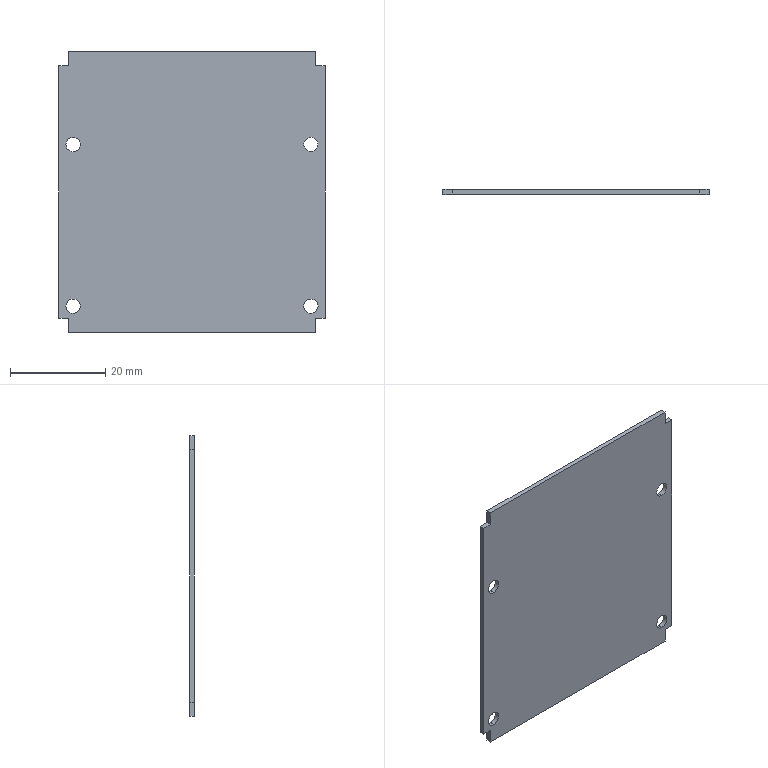Part | NX | features BREP 1 | 1 solid | 22 faces | box 56 x 1 x 59 mm | volume 3252 mm3 | plane 14 | cylinder 8 | commonest cylinder face diameters 3 x8
STEP:
#1=CARTESIAN_POINT('',(25.,1.,8.5));
#2=VERTEX_POINT('',#1);
#3=CARTESIAN_POINT('',(25.,1.,11.5));
#4=VERTEX_POINT('',#3);
#5=CARTESIAN_POINT('',(25.,1.,10.));
#6=DIRECTION('',(0.,1.,0.));
#7=DIRECTION('',(1.,0.,0.));
#8=AXIS2_PLACEMENT_3D('',#5,#6,#7);
#9=CIRCLE('',#8,1.5);
#10=EDGE_CURVE('',#2,#4,#9,.T.);
#11=ORIENTED_EDGE('',*,*,#10,.T.);
#12=CARTESIAN_POINT('',(25.,0.,11.5));
#13=VERTEX_POINT('',#12);
#14=CARTESIAN_POINT('',(25.,1.,11.5));
#15=DIRECTION('',(0.,1.,0.));
#16=VECTOR('',#15,1000.);
#17=LINE('',#14,#16);
#18=EDGE_CURVE('',#13,#4,#17,.T.);
#19=ORIENTED_EDGE('',*,*,#18,.F.);
#20=CARTESIAN_POINT('',(25.,0.,8.5));
#21=VERTEX_POINT('',#20);
#22=CARTESIAN_POINT('',(25.,0.,10.));
#23=DIRECTION('',(0.,1.,0.));
#24=DIRECTION('',(1.,0.,0.));
#25=AXIS2_PLACEMENT_3D('',#22,#23,#24);
#26=CIRCLE('',#25,1.5);
#27=EDGE_CURVE('',#21,#13,#26,.T.);
#28=ORIENTED_EDGE('',*,*,#27,.F.);
#29=CARTESIAN_POINT('',(25.,1.,8.5));
#30=DIRECTION('',(0.,1.,0.));
#31=VECTOR('',#30,1000.);
#32=LINE('',#29,#31);
#33=EDGE_CURVE('',#21,#2,#32,.T.);
#34=ORIENTED_EDGE('',*,*,#33,.T.);
#35=EDGE_LOOP('',(#11,#19,#28,#34));
#36=FACE_BOUND('',#35,.T.);
#37=CARTESIAN_POINT('',(25.,1.,10.));
#38=DIRECTION('',(0.,-1.,0.));
#39=DIRECTION('',(0.,0.,-1.));
#40=AXIS2_PLACEMENT_3D('',#37,#38,#39);
#41=CYLINDRICAL_SURFACE('',#40,1.5);
#42=ADVANCED_FACE('',(#36),#41,.F.);
#43=CARTESIAN_POINT('',(28.,1.,26.5));
#44=VERTEX_POINT('',#43);
#45=CARTESIAN_POINT('',(28.,1.,-26.5));
#46=VERTEX_POINT('',#45);
#47=CARTESIAN_POINT('',(28.,1.,0.));
#48=DIRECTION('',(0.,0.,-1.));
#49=VECTOR('',#48,1000.);
#50=LINE('',#47,#49);
#51=EDGE_CURVE('',#44,#46,#50,.T.);
#52=ORIENTED_EDGE('',*,*,#51,.T.);
#53=CARTESIAN_POINT('',(26.,1.,-26.5));
#54=VERTEX_POINT('',#53);
#55=CARTESIAN_POINT('',(27.,1.,-26.5));
#56=DIRECTION('',(-1.,0.,0.));
#57=VECTOR('',#56,1000.);
#58=LINE('',#55,#57);
#59=EDGE_CURVE('',#46,#54,#58,.T.);
#60=ORIENTED_EDGE('',*,*,#59,.T.);
#61=CARTESIAN_POINT('',(26.,1.,-29.5));
#62=VERTEX_POINT('',#61);
#63=CARTESIAN_POINT('',(26.,1.,-28.));
#64=DIRECTION('',(0.,0.,-1.));
#65=VECTOR('',#64,1000.);
#66=LINE('',#63,#65);
#67=EDGE_CURVE('',#54,#62,#66,.T.);
#68=ORIENTED_EDGE('',*,*,#67,.T.);
#69=CARTESIAN_POINT('',(-26.,1.,-29.5));
#70=VERTEX_POINT('',#69);
#71=CARTESIAN_POINT('',(0.,1.,-29.5));
#72=DIRECTION('',(-1.,0.,0.));
#73=VECTOR('',#72,1000.);
#74=LINE('',#71,#73);
#75=EDGE_CURVE('',#62,#70,#74,.T.);
#76=ORIENTED_EDGE('',*,*,#75,.T.);
#77=CARTESIAN_POINT('',(-26.,1.,-26.5));
#78=VERTEX_POINT('',#77);
#79=CARTESIAN_POINT('',(-26.,1.,-28.));
#80=DIRECTION('',(0.,0.,1.));
#81=VECTOR('',#80,1000.);
#82=LINE('',#79,#81);
#83=EDGE_CURVE('',#70,#78,#82,.T.);
#84=ORIENTED_EDGE('',*,*,#83,.T.);
#85=CARTESIAN_POINT('',(-28.,1.,-26.5));
#86=VERTEX_POINT('',#85);
#87=CARTESIAN_POINT('',(-27.,1.,-26.5));
#88=DIRECTION('',(-1.,0.,0.));
#89=VECTOR('',#88,1000.);
#90=LINE('',#87,#89);
#91=EDGE_CURVE('',#78,#86,#90,.T.);
#92=ORIENTED_EDGE('',*,*,#91,.T.);
#93=CARTESIAN_POINT('',(-28.,1.,26.5));
#94=VERTEX_POINT('',#93);
#95=CARTESIAN_POINT('',(-28.,1.,0.));
#96=DIRECTION('',(0.,0.,1.));
#97=VECTOR('',#96,1000.);
#98=LINE('',#95,#97);
#99=EDGE_CURVE('',#86,#94,#98,.T.);
#100=ORIENTED_EDGE('',*,*,#99,.T.);
#101=CARTESIAN_POINT('',(-26.,1.,26.5));
#102=VERTEX_POINT('',#101);
#103=CARTESIAN_POINT('',(-27.,1.,26.5));
#104=DIRECTION('',(1.,0.,0.));
#105=VECTOR('',#104,1000.);
#106=LINE('',#103,#105);
#107=EDGE_CURVE('',#94,#102,#106,.T.);
#108=ORIENTED_EDGE('',*,*,#107,.T.);
#109=CARTESIAN_POINT('',(-26.,1.,29.5));
#110=VERTEX_POINT('',#109);
#111=CARTESIAN_POINT('',(-26.,1.,28.));
#112=DIRECTION('',(0.,0.,1.));
#113=VECTOR('',#112,1000.);
#114=LINE('',#111,#113);
#115=EDGE_CURVE('',#102,#110,#114,.T.);
#116=ORIENTED_EDGE('',*,*,#115,.T.);
#117=CARTESIAN_POINT('',(26.,1.,29.5));
#118=VERTEX_POINT('',#117);
#119=CARTESIAN_POINT('',(0.,1.,29.5));
#120=DIRECTION('',(1.,0.,0.));
#121=VECTOR('',#120,1000.);
#122=LINE('',#119,#121);
#123=EDGE_CURVE('',#110,#118,#122,.T.);
#124=ORIENTED_EDGE('',*,*,#123,.T.);
#125=CARTESIAN_POINT('',(26.,1.,26.5));
#126=VERTEX_POINT('',#125);
#127=CARTESIAN_POINT('',(26.,1.,28.));
#128=DIRECTION('',(0.,0.,-1.));
#129=VECTOR('',#128,1000.);
#130=LINE('',#127,#129);
#131=EDGE_CURVE('',#118,#126,#130,.T.);
#132=ORIENTED_EDGE('',*,*,#131,.T.);
#133=CARTESIAN_POINT('',(27.,1.,26.5));
#134=DIRECTION('',(1.,0.,0.));
#135=VECTOR('',#134,1000.);
#136=LINE('',#133,#135);
#137=EDGE_CURVE('',#126,#44,#136,.T.);
#138=ORIENTED_EDGE('',*,*,#137,.T.);
#139=EDGE_LOOP('',(#52,#60,#68,#76,#84,#92,#100,#108,#116,#124,#132,#138));
#140=FACE_BOUND('',#139,.T.);
#141=CARTESIAN_POINT('',(-25.,1.,-25.5));
#142=VERTEX_POINT('',#141);
#143=CARTESIAN_POINT('',(-25.,1.,-22.5));
#144=VERTEX_POINT('',#143);
#145=CARTESIAN_POINT('',(-25.,1.,-25.5));
#146=CARTESIAN_POINT('',(-25.18,1.,-25.5));
#147=CARTESIAN_POINT('',(-25.36,1.,-25.473));
#148=CARTESIAN_POINT('',(-25.535,1.,-25.419));
#149=CARTESIAN_POINT('',(-25.862,1.,-25.26));
#150=CARTESIAN_POINT('',(-26.129,1.,-25.012));
#151=CARTESIAN_POINT('',(-26.242,1.,-24.869));
#152=CARTESIAN_POINT('',(-26.423,1.,-24.553));
#153=CARTESIAN_POINT('',(-26.503,1.,-24.198));
#154=CARTESIAN_POINT('',(-26.516,1.,-24.016));
#155=CARTESIAN_POINT('',(-26.487,1.,-23.653));
#156=CARTESIAN_POINT('',(-26.353,1.,-23.315));
#157=CARTESIAN_POINT('',(-26.26,1.,-23.157));
#158=CARTESIAN_POINT('',(-26.031,1.,-22.874));
#159=CARTESIAN_POINT('',(-25.73,1.,-22.671));
#160=CARTESIAN_POINT('',(-25.564,1.,-22.593));
#161=CARTESIAN_POINT('',(-25.349,1.,-22.528));
#162=CARTESIAN_POINT('',(-25.127,1.,-22.505));
#163=CARTESIAN_POINT('',(-25.085,1.,-22.502));
#164=CARTESIAN_POINT('',(-25.042,1.,-22.5));
#165=CARTESIAN_POINT('',(-25.,1.,-22.5));
#166=B_SPLINE_CURVE_WITH_KNOTS('',5,(#145,#146,#147,#148,#149,#150,#151,#152,#153,#154,#155,#156,#157,#158,#159,#160,#161,#162,#163,#164,#165),.UNSPECIFIED.,.F.,.F.,(6,3,3,3,3,3,6),(0.,0.191,0.382,0.573,0.764,0.9549,1.),.UNSPECIFIED.);
#167=EDGE_CURVE('',#142,#144,#166,.T.);
#168=ORIENTED_EDGE('',*,*,#167,.F.);
#169=CARTESIAN_POINT('',(-25.,1.,-22.5));
#170=CARTESIAN_POINT('',(-24.82,1.,-22.5));
#171=CARTESIAN_POINT('',(-24.64,1.,-22.527));
#172=CARTESIAN_POINT('',(-24.465,1.,-22.581));
#173=CARTESIAN_POINT('',(-24.138,1.,-22.74));
#174=CARTESIAN_POINT('',(-23.871,1.,-22.988));
#175=CARTESIAN_POINT('',(-23.758,1.,-23.131));
#176=CARTESIAN_POINT('',(-23.577,1.,-23.447));
#177=CARTESIAN_POINT('',(-23.497,1.,-23.802));
#178=CARTESIAN_POINT('',(-23.484,1.,-23.984));
#179=CARTESIAN_POINT('',(-23.513,1.,-24.347));
#180=CARTESIAN_POINT('',(-23.647,1.,-24.685));
#181=CARTESIAN_POINT('',(-23.74,1.,-24.843));
#182=CARTESIAN_POINT('',(-23.969,1.,-25.126));
#183=CARTESIAN_POINT('',(-24.27,1.,-25.329));
#184=CARTESIAN_POINT('',(-24.436,1.,-25.407));
#185=CARTESIAN_POINT('',(-24.651,1.,-25.472));
#186=CARTESIAN_POINT('',(-24.873,1.,-25.495));
#187=CARTESIAN_POINT('',(-24.915,1.,-25.498));
#188=CARTESIAN_POINT('',(-24.958,1.,-25.5));
#189=CARTESIAN_POINT('',(-25.,1.,-25.5));
#190=B_SPLINE_CURVE_WITH_KNOTS('',5,(#169,#170,#171,#172,#173,#174,#175,#176,#177,#178,#179,#180,#181,#182,#183,#184,#185,#186,#187,#188,#189),.UNSPECIFIED.,.F.,.F.,(6,3,3,3,3,3,6),(0.,0.191,0.382,0.573,0.764,0.9549,1.),.UNSPECIFIED.);
#191=EDGE_CURVE('',#144,#142,#190,.T.);
#192=ORIENTED_EDGE('',*,*,#191,.F.);
#193=EDGE_LOOP('',(#168,#192));
#194=FACE_BOUND('',#193,.T.);
#195=CARTESIAN_POINT('',(25.,1.,-25.5));
#196=VERTEX_POINT('',#195);
#197=CARTESIAN_POINT('',(25.,1.,-22.5));
#198=VERTEX_POINT('',#197);
#199=CARTESIAN_POINT('',(25.,1.,-25.5));
#200=CARTESIAN_POINT('',(24.82,1.,-25.5));
#201=CARTESIAN_POINT('',(24.64,1.,-25.473));
#202=CARTESIAN_POINT('',(24.465,1.,-25.419));
#203=CARTESIAN_POINT('',(24.138,1.,-25.26));
#204=CARTESIAN_POINT('',(23.871,1.,-25.012));
#205=CARTESIAN_POINT('',(23.758,1.,-24.869));
#206=CARTESIAN_POINT('',(23.577,1.,-24.553));
#207=CARTESIAN_POINT('',(23.497,1.,-24.198));
#208=CARTESIAN_POINT('',(23.484,1.,-24.016));
#209=CARTESIAN_POINT('',(23.513,1.,-23.653));
#210=CARTESIAN_POINT('',(23.647,1.,-23.315));
#211=CARTESIAN_POINT('',(23.74,1.,-23.157));
#212=CARTESIAN_POINT('',(23.969,1.,-22.874));
#213=CARTESIAN_POINT('',(24.27,1.,-22.671));
#214=CARTESIAN_POINT('',(24.436,1.,-22.593));
#215=CARTESIAN_POINT('',(24.651,1.,-22.528));
#216=CARTESIAN_POINT('',(24.873,1.,-22.505));
#217=CARTESIAN_POINT('',(24.915,1.,-22.502));
#218=CARTESIAN_POINT('',(24.958,1.,-22.5));
#219=CARTESIAN_POINT('',(25.,1.,-22.5));
#220=B_SPLINE_CURVE_WITH_KNOTS('',5,(#199,#200,#201,#202,#203,#204,#205,#206,#207,#208,#209,#210,#211,#212,#213,#214,#215,#216,#217,#218,#219),.UNSPECIFIED.,.F.,.F.,(6,3,3,3,3,3,6),(0.,0.191,0.382,0.573,0.764,0.9549,1.),.UNSPECIFIED.);
#221=EDGE_CURVE('',#196,#198,#220,.T.);
#222=ORIENTED_EDGE('',*,*,#221,.F.);
#223=CARTESIAN_POINT('',(25.,1.,-22.5));
#224=CARTESIAN_POINT('',(25.18,1.,-22.5));
#225=CARTESIAN_POINT('',(25.36,1.,-22.527));
#226=CARTESIAN_POINT('',(25.535,1.,-22.581));
#227=CARTESIAN_POINT('',(25.862,1.,-22.74));
#228=CARTESIAN_POINT('',(26.129,1.,-22.988));
#229=CARTESIAN_POINT('',(26.242,1.,-23.131));
#230=CARTESIAN_POINT('',(26.423,1.,-23.447));
#231=CARTESIAN_POINT('',(26.503,1.,-23.802));
#232=CARTESIAN_POINT('',(26.516,1.,-23.984));
#233=CARTESIAN_POINT('',(26.487,1.,-24.347));
#234=CARTESIAN_POINT('',(26.353,1.,-24.685));
#235=CARTESIAN_POINT('',(26.26,1.,-24.843));
#236=CARTESIAN_POINT('',(26.031,1.,-25.126));
#237=CARTESIAN_POINT('',(25.73,1.,-25.329));
#238=CARTESIAN_POINT('',(25.564,1.,-25.407));
#239=CARTESIAN_POINT('',(25.349,1.,-25.472));
#240=CARTESIAN_POINT('',(25.127,1.,-25.495));
#241=CARTESIAN_POINT('',(25.085,1.,-25.498));
#242=CARTESIAN_POINT('',(25.042,1.,-25.5));
#243=CARTESIAN_POINT('',(25.,1.,-25.5));
#244=B_SPLINE_CURVE_WITH_KNOTS('',5,(#223,#224,#225,#226,#227,#228,#229,#230,#231,#232,#233,#234,#235,#236,#237,#238,#239,#240,#241,#242,#243),.UNSPECIFIED.,.F.,.F.,(6,3,3,3,3,3,6),(0.,0.191,0.382,0.573,0.764,0.9549,1.),.UNSPECIFIED.);
#245=EDGE_CURVE('',#198,#196,#244,.T.);
#246=ORIENTED_EDGE('',*,*,#245,.F.);
#247=EDGE_LOOP('',(#222,#246));
#248=FACE_BOUND('',#247,.T.);
#249=CARTESIAN_POINT('',(-25.,1.,8.5));
#250=VERTEX_POINT('',#249);
#251=CARTESIAN_POINT('',(-25.,1.,11.5));
#252=VERTEX_POINT('',#251);
#253=CARTESIAN_POINT('',(-25.,1.,8.5));
#254=CARTESIAN_POINT('',(-25.18,1.,8.5));
#255=CARTESIAN_POINT('',(-25.36,1.,8.527));
#256=CARTESIAN_POINT('',(-25.535,1.,8.581));
#257=CARTESIAN_POINT('',(-25.862,1.,8.74));
#258=CARTESIAN_POINT('',(-26.129,1.,8.988));
#259=CARTESIAN_POINT('',(-26.242,1.,9.131));
#260=CARTESIAN_POINT('',(-26.423,1.,9.447));
#261=CARTESIAN_POINT('',(-26.503,1.,9.802));
#262=CARTESIAN_POINT('',(-26.516,1.,9.984));
#263=CARTESIAN_POINT('',(-26.487,1.,10.347));
#264=CARTESIAN_POINT('',(-26.353,1.,10.685));
#265=CARTESIAN_POINT('',(-26.26,1.,10.843));
#266=CARTESIAN_POINT('',(-26.031,1.,11.126));
#267=CARTESIAN_POINT('',(-25.73,1.,11.329));
#268=CARTESIAN_POINT('',(-25.564,1.,11.407));
#269=CARTESIAN_POINT('',(-25.349,1.,11.472));
#270=CARTESIAN_POINT('',(-25.127,1.,11.495));
#271=CARTESIAN_POINT('',(-25.085,1.,11.498));
#272=CARTESIAN_POINT('',(-25.042,1.,11.5));
#273=CARTESIAN_POINT('',(-25.,1.,11.5));
#274=B_SPLINE_CURVE_WITH_KNOTS('',5,(#253,#254,#255,#256,#257,#258,#259,#260,#261,#262,#263,#264,#265,#266,#267,#268,#269,#270,#271,#272,#273),.UNSPECIFIED.,.F.,.F.,(6,3,3,3,3,3,6),(0.,0.191,0.382,0.573,0.764,0.9549,1.),.UNSPECIFIED.);
#275=EDGE_CURVE('',#250,#252,#274,.T.);
#276=ORIENTED_EDGE('',*,*,#275,.F.);
#277=CARTESIAN_POINT('',(-25.,1.,11.5));
#278=CARTESIAN_POINT('',(-24.82,1.,11.5));
#279=CARTESIAN_POINT('',(-24.64,1.,11.473));
#280=CARTESIAN_POINT('',(-24.465,1.,11.419));
#281=CARTESIAN_POINT('',(-24.138,1.,11.26));
#282=CARTESIAN_POINT('',(-23.871,1.,11.012));
#283=CARTESIAN_POINT('',(-23.758,1.,10.869));
#284=CARTESIAN_POINT('',(-23.577,1.,10.553));
#285=CARTESIAN_POINT('',(-23.497,1.,10.198));
#286=CARTESIAN_POINT('',(-23.484,1.,10.016));
#287=CARTESIAN_POINT('',(-23.513,1.,9.653));
#288=CARTESIAN_POINT('',(-23.647,1.,9.315));
#289=CARTESIAN_POINT('',(-23.74,1.,9.157));
#290=CARTESIAN_POINT('',(-23.969,1.,8.874));
#291=CARTESIAN_POINT('',(-24.27,1.,8.671));
#292=CARTESIAN_POINT('',(-24.436,1.,8.593));
#293=CARTESIAN_POINT('',(-24.651,1.,8.528));
#294=CARTESIAN_POINT('',(-24.873,1.,8.505));
#295=CARTESIAN_POINT('',(-24.915,1.,8.502));
#296=CARTESIAN_POINT('',(-24.958,1.,8.5));
#297=CARTESIAN_POINT('',(-25.,1.,8.5));
#298=B_SPLINE_CURVE_WITH_KNOTS('',5,(#277,#278,#279,#280,#281,#282,#283,#284,#285,#286,#287,#288,#289,#290,#291,#292,#293,#294,#295,#296,#297),.UNSPECIFIED.,.F.,.F.,(6,3,3,3,3,3,6),(0.,0.191,0.382,0.573,0.764,0.9549,1.),.UNSPECIFIED.);
#299=EDGE_CURVE('',#252,#250,#298,.T.);
#300=ORIENTED_EDGE('',*,*,#299,.F.);
#301=EDGE_LOOP('',(#276,#300));
#302=FACE_BOUND('',#301,.T.);
#303=ORIENTED_EDGE('',*,*,#10,.F.);
#304=CARTESIAN_POINT('',(25.,1.,11.5));
#305=CARTESIAN_POINT('',(25.18,1.,11.5));
#306=CARTESIAN_POINT('',(25.36,1.,11.473));
#307=CARTESIAN_POINT('',(25.535,1.,11.419));
#308=CARTESIAN_POINT('',(25.862,1.,11.26));
#309=CARTESIAN_POINT('',(26.129,1.,11.012));
#310=CARTESIAN_POINT('',(26.242,1.,10.869));
#311=CARTESIAN_POINT('',(26.423,1.,10.553));
#312=CARTESIAN_POINT('',(26.503,1.,10.198));
#313=CARTESIAN_POINT('',(26.516,1.,10.016));
#314=CARTESIAN_POINT('',(26.487,1.,9.653));
#315=CARTESIAN_POINT('',(26.353,1.,9.315));
#316=CARTESIAN_POINT('',(26.26,1.,9.157));
#317=CARTESIAN_POINT('',(26.031,1.,8.874));
#318=CARTESIAN_POINT('',(25.73,1.,8.671));
#319=CARTESIAN_POINT('',(25.564,1.,8.593));
#320=CARTESIAN_POINT('',(25.349,1.,8.528));
#321=CARTESIAN_POINT('',(25.127,1.,8.505));
#322=CARTESIAN_POINT('',(25.085,1.,8.502));
#323=CARTESIAN_POINT('',(25.042,1.,8.5));
#324=CARTESIAN_POINT('',(25.,1.,8.5));
#325=B_SPLINE_CURVE_WITH_KNOTS('',5,(#304,#305,#306,#307,#308,#309,#310,#311,#312,#313,#314,#315,#316,#317,#318,#319,#320,#321,#322,#323,#324),.UNSPECIFIED.,.F.,.F.,(6,3,3,3,3,3,6),(0.,0.191,0.382,0.573,0.764,0.9549,1.),.UNSPECIFIED.);
#326=EDGE_CURVE('',#4,#2,#325,.T.);
#327=ORIENTED_EDGE('',*,*,#326,.F.);
#328=EDGE_LOOP('',(#303,#327));
#329=FACE_BOUND('',#328,.T.);
#330=CARTESIAN_POINT('',(0.,1.,0.));
#331=DIRECTION('',(0.,-1.,0.));
#332=DIRECTION('',(0.,0.,1.));
#333=AXIS2_PLACEMENT_3D('',#330,#331,#332);
#334=PLANE('',#333);
#335=ADVANCED_FACE('',(#140,#194,#248,#302,#329),#334,.F.);
#336=ORIENTED_EDGE('',*,*,#18,.T.);
#337=ORIENTED_EDGE('',*,*,#326,.T.);
#338=ORIENTED_EDGE('',*,*,#33,.F.);
#339=CARTESIAN_POINT('',(25.,0.,10.));
#340=DIRECTION('',(0.,1.,0.));
#341=DIRECTION('',(1.,0.,0.));
#342=AXIS2_PLACEMENT_3D('',#339,#340,#341);
#343=CIRCLE('',#342,1.5);
#344=EDGE_CURVE('',#13,#21,#343,.T.);
#345=ORIENTED_EDGE('',*,*,#344,.F.);
#346=EDGE_LOOP('',(#336,#337,#338,#345));
#347=FACE_BOUND('',#346,.T.);
#348=CARTESIAN_POINT('',(25.,1.,10.));
#349=DIRECTION('',(0.,-1.,0.));
#350=DIRECTION('',(0.,0.,1.));
#351=AXIS2_PLACEMENT_3D('',#348,#349,#350);
#352=CYLINDRICAL_SURFACE('',#351,1.5);
#353=ADVANCED_FACE('',(#347),#352,.F.);
#354=CARTESIAN_POINT('',(28.,0.,26.5));
#355=VERTEX_POINT('',#354);
#356=CARTESIAN_POINT('',(28.,0.,-26.5));
#357=VERTEX_POINT('',#356);
#358=CARTESIAN_POINT('',(28.,0.,0.));
#359=DIRECTION('',(0.,0.,-1.));
#360=VECTOR('',#359,1000.);
#361=LINE('',#358,#360);
#362=EDGE_CURVE('',#355,#357,#361,.T.);
#363=ORIENTED_EDGE('',*,*,#362,.F.);
#364=CARTESIAN_POINT('',(26.,0.,26.5));
#365=VERTEX_POINT('',#364);
#366=CARTESIAN_POINT('',(27.,0.,26.5));
#367=DIRECTION('',(1.,0.,0.));
#368=VECTOR('',#367,1000.);
#369=LINE('',#366,#368);
#370=EDGE_CURVE('',#365,#355,#369,.T.);
#371=ORIENTED_EDGE('',*,*,#370,.F.);
#372=CARTESIAN_POINT('',(26.,0.,29.5));
#373=VERTEX_POINT('',#372);
#374=CARTESIAN_POINT('',(26.,0.,28.));
#375=DIRECTION('',(0.,0.,-1.));
#376=VECTOR('',#375,1000.);
#377=LINE('',#374,#376);
#378=EDGE_CURVE('',#373,#365,#377,.T.);
#379=ORIENTED_EDGE('',*,*,#378,.F.);
#380=CARTESIAN_POINT('',(-26.,0.,29.5));
#381=VERTEX_POINT('',#380);
#382=CARTESIAN_POINT('',(0.,0.,29.5));
#383=DIRECTION('',(1.,0.,0.));
#384=VECTOR('',#383,1000.);
#385=LINE('',#382,#384);
#386=EDGE_CURVE('',#381,#373,#385,.T.);
#387=ORIENTED_EDGE('',*,*,#386,.F.);
#388=CARTESIAN_POINT('',(-26.,0.,26.5));
#389=VERTEX_POINT('',#388);
#390=CARTESIAN_POINT('',(-26.,0.,28.));
#391=DIRECTION('',(0.,0.,1.));
#392=VECTOR('',#391,1000.);
#393=LINE('',#390,#392);
#394=EDGE_CURVE('',#389,#381,#393,.T.);
#395=ORIENTED_EDGE('',*,*,#394,.F.);
#396=CARTESIAN_POINT('',(-28.,0.,26.5));
#397=VERTEX_POINT('',#396);
#398=CARTESIAN_POINT('',(-27.,0.,26.5));
#399=DIRECTION('',(1.,0.,0.));
#400=VECTOR('',#399,1000.);
#401=LINE('',#398,#400);
#402=EDGE_CURVE('',#397,#389,#401,.T.);
#403=ORIENTED_EDGE('',*,*,#402,.F.);
#404=CARTESIAN_POINT('',(-28.,0.,-26.5));
#405=VERTEX_POINT('',#404);
#406=CARTESIAN_POINT('',(-28.,0.,0.));
#407=DIRECTION('',(0.,0.,1.));
#408=VECTOR('',#407,1000.);
#409=LINE('',#406,#408);
#410=EDGE_CURVE('',#405,#397,#409,.T.);
#411=ORIENTED_EDGE('',*,*,#410,.F.);
#412=CARTESIAN_POINT('',(-26.,0.,-26.5));
#413=VERTEX_POINT('',#412);
#414=CARTESIAN_POINT('',(-27.,0.,-26.5));
#415=DIRECTION('',(-1.,0.,0.));
#416=VECTOR('',#415,1000.);
#417=LINE('',#414,#416);
#418=EDGE_CURVE('',#413,#405,#417,.T.);
#419=ORIENTED_EDGE('',*,*,#418,.F.);
#420=CARTESIAN_POINT('',(-26.,0.,-29.5));
#421=VERTEX_POINT('',#420);
#422=CARTESIAN_POINT('',(-26.,0.,-28.));
#423=DIRECTION('',(0.,0.,1.));
#424=VECTOR('',#423,1000.);
#425=LINE('',#422,#424);
#426=EDGE_CURVE('',#421,#413,#425,.T.);
#427=ORIENTED_EDGE('',*,*,#426,.F.);
#428=CARTESIAN_POINT('',(26.,0.,-29.5));
#429=VERTEX_POINT('',#428);
#430=CARTESIAN_POINT('',(0.,0.,-29.5));
#431=DIRECTION('',(-1.,0.,0.));
#432=VECTOR('',#431,1000.);
#433=LINE('',#430,#432);
#434=EDGE_CURVE('',#429,#421,#433,.T.);
#435=ORIENTED_EDGE('',*,*,#434,.F.);
#436=CARTESIAN_POINT('',(26.,0.,-26.5));
#437=VERTEX_POINT('',#436);
#438=CARTESIAN_POINT('',(26.,0.,-28.));
#439=DIRECTION('',(0.,0.,-1.));
#440=VECTOR('',#439,1000.);
#441=LINE('',#438,#440);
#442=EDGE_CURVE('',#437,#429,#441,.T.);
#443=ORIENTED_EDGE('',*,*,#442,.F.);
#444=CARTESIAN_POINT('',(27.,0.,-26.5));
#445=DIRECTION('',(-1.,0.,0.));
#446=VECTOR('',#445,1000.);
#447=LINE('',#444,#446);
#448=EDGE_CURVE('',#357,#437,#447,.T.);
#449=ORIENTED_EDGE('',*,*,#448,.F.);
#450=EDGE_LOOP('',(#363,#371,#379,#387,#395,#403,#411,#419,#427,#435,#443,#449));
#451=FACE_BOUND('',#450,.T.);
#452=CARTESIAN_POINT('',(-25.,0.,8.5));
#453=VERTEX_POINT('',#452);
#454=CARTESIAN_POINT('',(-25.,0.,11.5));
#455=VERTEX_POINT('',#454);
#456=CARTESIAN_POINT('',(-25.,0.,8.5));
#457=CARTESIAN_POINT('',(-25.18,0.,8.5));
#458=CARTESIAN_POINT('',(-25.36,0.,8.527));
#459=CARTESIAN_POINT('',(-25.535,0.,8.581));
#460=CARTESIAN_POINT('',(-25.862,0.,8.74));
#461=CARTESIAN_POINT('',(-26.129,0.,8.988));
#462=CARTESIAN_POINT('',(-26.242,0.,9.131));
#463=CARTESIAN_POINT('',(-26.423,0.,9.447));
#464=CARTESIAN_POINT('',(-26.503,0.,9.802));
#465=CARTESIAN_POINT('',(-26.516,0.,9.984));
#466=CARTESIAN_POINT('',(-26.487,0.,10.347));
#467=CARTESIAN_POINT('',(-26.353,0.,10.685));
#468=CARTESIAN_POINT('',(-26.26,0.,10.843));
#469=CARTESIAN_POINT('',(-26.031,0.,11.126));
#470=CARTESIAN_POINT('',(-25.73,0.,11.329));
#471=CARTESIAN_POINT('',(-25.564,0.,11.407));
#472=CARTESIAN_POINT('',(-25.349,0.,11.472));
#473=CARTESIAN_POINT('',(-25.127,0.,11.495));
#474=CARTESIAN_POINT('',(-25.085,0.,11.498));
#475=CARTESIAN_POINT('',(-25.042,0.,11.5));
#476=CARTESIAN_POINT('',(-25.,0.,11.5));
#477=B_SPLINE_CURVE_WITH_KNOTS('',5,(#456,#457,#458,#459,#460,#461,#462,#463,#464,#465,#466,#467,#468,#469,#470,#471,#472,#473,#474,#475,#476),.UNSPECIFIED.,.F.,.F.,(6,3,3,3,3,3,6),(0.,0.191,0.382,0.573,0.764,0.9549,1.),.UNSPECIFIED.);
#478=EDGE_CURVE('',#453,#455,#477,.T.);
#479=ORIENTED_EDGE('',*,*,#478,.T.);
#480=CARTESIAN_POINT('',(-25.,0.,11.5));
#481=CARTESIAN_POINT('',(-24.82,0.,11.5));
#482=CARTESIAN_POINT('',(-24.64,0.,11.473));
#483=CARTESIAN_POINT('',(-24.465,0.,11.419));
#484=CARTESIAN_POINT('',(-24.138,0.,11.26));
#485=CARTESIAN_POINT('',(-23.871,0.,11.012));
#486=CARTESIAN_POINT('',(-23.758,0.,10.869));
#487=CARTESIAN_POINT('',(-23.577,0.,10.553));
#488=CARTESIAN_POINT('',(-23.497,0.,10.198));
#489=CARTESIAN_POINT('',(-23.484,0.,10.016));
#490=CARTESIAN_POINT('',(-23.513,0.,9.653));
#491=CARTESIAN_POINT('',(-23.647,0.,9.315));
#492=CARTESIAN_POINT('',(-23.74,0.,9.157));
#493=CARTESIAN_POINT('',(-23.969,0.,8.874));
#494=CARTESIAN_POINT('',(-24.27,0.,8.671));
#495=CARTESIAN_POINT('',(-24.436,0.,8.593));
#496=CARTESIAN_POINT('',(-24.651,0.,8.528));
#497=CARTESIAN_POINT('',(-24.873,0.,8.505));
#498=CARTESIAN_POINT('',(-24.915,0.,8.502));
#499=CARTESIAN_POINT('',(-24.958,0.,8.5));
#500=CARTESIAN_POINT('',(-25.,0.,8.5));
#501=B_SPLINE_CURVE_WITH_KNOTS('',5,(#480,#481,#482,#483,#484,#485,#486,#487,#488,#489,#490,#491,#492,#493,#494,#495,#496,#497,#498,#499,#500),.UNSPECIFIED.,.F.,.F.,(6,3,3,3,3,3,6),(0.,0.191,0.382,0.573,0.764,0.9549,1.),.UNSPECIFIED.);
#502=EDGE_CURVE('',#455,#453,#501,.T.);
#503=ORIENTED_EDGE('',*,*,#502,.T.);
#504=EDGE_LOOP('',(#479,#503));
#505=FACE_BOUND('',#504,.T.);
#506=CARTESIAN_POINT('',(-25.,0.,-25.5));
#507=VERTEX_POINT('',#506);
#508=CARTESIAN_POINT('',(-25.,0.,-22.5));
#509=VERTEX_POINT('',#508);
#510=CARTESIAN_POINT('',(-25.,0.,-25.5));
#511=CARTESIAN_POINT('',(-25.18,0.,-25.5));
#512=CARTESIAN_POINT('',(-25.36,0.,-25.473));
#513=CARTESIAN_POINT('',(-25.535,0.,-25.419));
#514=CARTESIAN_POINT('',(-25.862,0.,-25.26));
#515=CARTESIAN_POINT('',(-26.129,0.,-25.012));
#516=CARTESIAN_POINT('',(-26.242,0.,-24.869));
#517=CARTESIAN_POINT('',(-26.423,0.,-24.553));
#518=CARTESIAN_POINT('',(-26.503,0.,-24.198));
#519=CARTESIAN_POINT('',(-26.516,0.,-24.016));
#520=CARTESIAN_POINT('',(-26.487,0.,-23.653));
#521=CARTESIAN_POINT('',(-26.353,0.,-23.315));
#522=CARTESIAN_POINT('',(-26.26,0.,-23.157));
#523=CARTESIAN_POINT('',(-26.031,0.,-22.874));
#524=CARTESIAN_POINT('',(-25.73,0.,-22.671));
#525=CARTESIAN_POINT('',(-25.564,0.,-22.593));
#526=CARTESIAN_POINT('',(-25.349,0.,-22.528));
#527=CARTESIAN_POINT('',(-25.127,0.,-22.505));
#528=CARTESIAN_POINT('',(-25.085,0.,-22.502));
#529=CARTESIAN_POINT('',(-25.042,0.,-22.5));
#530=CARTESIAN_POINT('',(-25.,0.,-22.5));
#531=B_SPLINE_CURVE_WITH_KNOTS('',5,(#510,#511,#512,#513,#514,#515,#516,#517,#518,#519,#520,#521,#522,#523,#524,#525,#526,#527,#528,#529,#530),.UNSPECIFIED.,.F.,.F.,(6,3,3,3,3,3,6),(0.,0.191,0.382,0.573,0.764,0.9549,1.),.UNSPECIFIED.);
#532=EDGE_CURVE('',#507,#509,#531,.T.);
#533=ORIENTED_EDGE('',*,*,#532,.T.);
#534=CARTESIAN_POINT('',(-25.,0.,-22.5));
#535=CARTESIAN_POINT('',(-24.82,0.,-22.5));
#536=CARTESIAN_POINT('',(-24.64,0.,-22.527));
#537=CARTESIAN_POINT('',(-24.465,0.,-22.581));
#538=CARTESIAN_POINT('',(-24.138,0.,-22.74));
#539=CARTESIAN_POINT('',(-23.871,0.,-22.988));
#540=CARTESIAN_POINT('',(-23.758,0.,-23.131));
#541=CARTESIAN_POINT('',(-23.577,0.,-23.447));
#542=CARTESIAN_POINT('',(-23.497,0.,-23.802));
#543=CARTESIAN_POINT('',(-23.484,0.,-23.984));
#544=CARTESIAN_POINT('',(-23.513,0.,-24.347));
#545=CARTESIAN_POINT('',(-23.647,0.,-24.685));
#546=CARTESIAN_POINT('',(-23.74,0.,-24.843));
#547=CARTESIAN_POINT('',(-23.969,0.,-25.126));
#548=CARTESIAN_POINT('',(-24.27,0.,-25.329));
#549=CARTESIAN_POINT('',(-24.436,0.,-25.407));
#550=CARTESIAN_POINT('',(-24.651,0.,-25.472));
#551=CARTESIAN_POINT('',(-24.873,0.,-25.495));
#552=CARTESIAN_POINT('',(-24.915,0.,-25.498));
#553=CARTESIAN_POINT('',(-24.958,0.,-25.5));
#554=CARTESIAN_POINT('',(-25.,0.,-25.5));
#555=B_SPLINE_CURVE_WITH_KNOTS('',5,(#534,#535,#536,#537,#538,#539,#540,#541,#542,#543,#544,#545,#546,#547,#548,#549,#550,#551,#552,#553,#554),.UNSPECIFIED.,.F.,.F.,(6,3,3,3,3,3,6),(0.,0.191,0.382,0.573,0.764,0.9549,1.),.UNSPECIFIED.);
#556=EDGE_CURVE('',#509,#507,#555,.T.);
#557=ORIENTED_EDGE('',*,*,#556,.T.);
#558=EDGE_LOOP('',(#533,#557));
#559=FACE_BOUND('',#558,.T.);
#560=CARTESIAN_POINT('',(25.,0.,-25.5));
#561=VERTEX_POINT('',#560);
#562=CARTESIAN_POINT('',(25.,0.,-22.5));
#563=VERTEX_POINT('',#562);
#564=CARTESIAN_POINT('',(25.,0.,-25.5));
#565=CARTESIAN_POINT('',(24.82,0.,-25.5));
#566=CARTESIAN_POINT('',(24.64,0.,-25.473));
#567=CARTESIAN_POINT('',(24.465,0.,-25.419));
#568=CARTESIAN_POINT('',(24.138,0.,-25.26));
#569=CARTESIAN_POINT('',(23.871,0.,-25.012));
#570=CARTESIAN_POINT('',(23.758,0.,-24.869));
#571=CARTESIAN_POINT('',(23.577,0.,-24.553));
#572=CARTESIAN_POINT('',(23.497,0.,-24.198));
#573=CARTESIAN_POINT('',(23.484,0.,-24.016));
#574=CARTESIAN_POINT('',(23.513,0.,-23.653));
#575=CARTESIAN_POINT('',(23.647,0.,-23.315));
#576=CARTESIAN_POINT('',(23.74,0.,-23.157));
#577=CARTESIAN_POINT('',(23.969,0.,-22.874));
#578=CARTESIAN_POINT('',(24.27,0.,-22.671));
#579=CARTESIAN_POINT('',(24.436,0.,-22.593));
#580=CARTESIAN_POINT('',(24.651,0.,-22.528));
#581=CARTESIAN_POINT('',(24.873,0.,-22.505));
#582=CARTESIAN_POINT('',(24.915,0.,-22.502));
#583=CARTESIAN_POINT('',(24.958,0.,-22.5));
#584=CARTESIAN_POINT('',(25.,0.,-22.5));
#585=B_SPLINE_CURVE_WITH_KNOTS('',5,(#564,#565,#566,#567,#568,#569,#570,#571,#572,#573,#574,#575,#576,#577,#578,#579,#580,#581,#582,#583,#584),.UNSPECIFIED.,.F.,.F.,(6,3,3,3,3,3,6),(0.,0.191,0.382,0.573,0.764,0.9549,1.),.UNSPECIFIED.);
#586=EDGE_CURVE('',#561,#563,#585,.T.);
#587=ORIENTED_EDGE('',*,*,#586,.T.);
#588=CARTESIAN_POINT('',(25.,0.,-22.5));
#589=CARTESIAN_POINT('',(25.18,0.,-22.5));
#590=CARTESIAN_POINT('',(25.36,0.,-22.527));
#591=CARTESIAN_POINT('',(25.535,0.,-22.581));
#592=CARTESIAN_POINT('',(25.862,0.,-22.74));
#593=CARTESIAN_POINT('',(26.129,0.,-22.988));
#594=CARTESIAN_POINT('',(26.242,0.,-23.131));
#595=CARTESIAN_POINT('',(26.423,0.,-23.447));
#596=CARTESIAN_POINT('',(26.503,0.,-23.802));
#597=CARTESIAN_POINT('',(26.516,0.,-23.984));
#598=CARTESIAN_POINT('',(26.487,0.,-24.347));
#599=CARTESIAN_POINT('',(26.353,0.,-24.685));
#600=CARTESIAN_POINT('',(26.26,0.,-24.843));
#601=CARTESIAN_POINT('',(26.031,0.,-25.126));
#602=CARTESIAN_POINT('',(25.73,0.,-25.329));
#603=CARTESIAN_POINT('',(25.564,0.,-25.407));
#604=CARTESIAN_POINT('',(25.349,0.,-25.472));
#605=CARTESIAN_POINT('',(25.127,0.,-25.495));
#606=CARTESIAN_POINT('',(25.085,0.,-25.498));
#607=CARTESIAN_POINT('',(25.042,0.,-25.5));
#608=CARTESIAN_POINT('',(25.,0.,-25.5));
#609=B_SPLINE_CURVE_WITH_KNOTS('',5,(#588,#589,#590,#591,#592,#593,#594,#595,#596,#597,#598,#599,#600,#601,#602,#603,#604,#605,#606,#607,#608),.UNSPECIFIED.,.F.,.F.,(6,3,3,3,3,3,6),(0.,0.191,0.382,0.573,0.764,0.9549,1.),.UNSPECIFIED.);
#610=EDGE_CURVE('',#563,#561,#609,.T.);
#611=ORIENTED_EDGE('',*,*,#610,.T.);
#612=EDGE_LOOP('',(#587,#611));
#613=FACE_BOUND('',#612,.T.);
#614=ORIENTED_EDGE('',*,*,#27,.T.);
#615=ORIENTED_EDGE('',*,*,#344,.T.);
#616=EDGE_LOOP('',(#614,#615));
#617=FACE_BOUND('',#616,.T.);
#618=CARTESIAN_POINT('',(0.,0.,0.));
#619=DIRECTION('',(0.,-1.,0.));
#620=DIRECTION('',(0.,0.,1.));
#621=AXIS2_PLACEMENT_3D('',#618,#619,#620);
#622=PLANE('',#621);
#623=ADVANCED_FACE('',(#451,#505,#559,#613,#617),#622,.T.);
#624=ORIENTED_EDGE('',*,*,#362,.T.);
#625=CARTESIAN_POINT('',(28.,0.5,-26.5));
#626=DIRECTION('',(0.,-1.,0.));
#627=VECTOR('',#626,1000.);
#628=LINE('',#625,#627);
#629=EDGE_CURVE('',#46,#357,#628,.T.);
#630=ORIENTED_EDGE('',*,*,#629,.F.);
#631=ORIENTED_EDGE('',*,*,#51,.F.);
#632=CARTESIAN_POINT('',(28.,0.5,26.5));
#633=DIRECTION('',(0.,-1.,0.));
#634=VECTOR('',#633,1000.);
#635=LINE('',#632,#634);
#636=EDGE_CURVE('',#44,#355,#635,.T.);
#637=ORIENTED_EDGE('',*,*,#636,.T.);
#638=EDGE_LOOP('',(#624,#630,#631,#637));
#639=FACE_BOUND('',#638,.T.);
#640=CARTESIAN_POINT('',(28.,1.,26.5));
#641=DIRECTION('',(-1.,0.,0.));
#642=DIRECTION('',(0.,0.,-1.));
#643=AXIS2_PLACEMENT_3D('',#640,#641,#642);
#644=PLANE('',#643);
#645=ADVANCED_FACE('',(#639),#644,.F.);
#646=ORIENTED_EDGE('',*,*,#448,.T.);
#647=CARTESIAN_POINT('',(26.,0.5,-26.5));
#648=DIRECTION('',(0.,-1.,0.));
#649=VECTOR('',#648,1000.);
#650=LINE('',#647,#649);
#651=EDGE_CURVE('',#54,#437,#650,.T.);
#652=ORIENTED_EDGE('',*,*,#651,.F.);
#653=ORIENTED_EDGE('',*,*,#59,.F.);
#654=ORIENTED_EDGE('',*,*,#629,.T.);
#655=EDGE_LOOP('',(#646,#652,#653,#654));
#656=FACE_BOUND('',#655,.T.);
#657=CARTESIAN_POINT('',(26.,1.,-26.5));
#658=DIRECTION('',(0.,0.,1.));
#659=DIRECTION('',(-1.,0.,0.));
#660=AXIS2_PLACEMENT_3D('',#657,#658,#659);
#661=PLANE('',#660);
#662=ADVANCED_FACE('',(#656),#661,.F.);
#663=ORIENTED_EDGE('',*,*,#442,.T.);
#664=CARTESIAN_POINT('',(26.,0.5,-29.5));
#665=DIRECTION('',(0.,-1.,0.));
#666=VECTOR('',#665,1000.);
#667=LINE('',#664,#666);
#668=EDGE_CURVE('',#62,#429,#667,.T.);
#669=ORIENTED_EDGE('',*,*,#668,.F.);
#670=ORIENTED_EDGE('',*,*,#67,.F.);
#671=ORIENTED_EDGE('',*,*,#651,.T.);
#672=EDGE_LOOP('',(#663,#669,#670,#671));
#673=FACE_BOUND('',#672,.T.);
#674=CARTESIAN_POINT('',(26.,1.,-29.5));
#675=DIRECTION('',(-1.,0.,0.));
#676=DIRECTION('',(0.,0.,-1.));
#677=AXIS2_PLACEMENT_3D('',#674,#675,#676);
#678=PLANE('',#677);
#679=ADVANCED_FACE('',(#673),#678,.F.);
#680=ORIENTED_EDGE('',*,*,#434,.T.);
#681=CARTESIAN_POINT('',(-26.,0.5,-29.5));
#682=DIRECTION('',(0.,-1.,0.));
#683=VECTOR('',#682,1000.);
#684=LINE('',#681,#683);
#685=EDGE_CURVE('',#70,#421,#684,.T.);
#686=ORIENTED_EDGE('',*,*,#685,.F.);
#687=ORIENTED_EDGE('',*,*,#75,.F.);
#688=ORIENTED_EDGE('',*,*,#668,.T.);
#689=EDGE_LOOP('',(#680,#686,#687,#688));
#690=FACE_BOUND('',#689,.T.);
#691=CARTESIAN_POINT('',(-26.,1.,-29.5));
#692=DIRECTION('',(0.,0.,1.));
#693=DIRECTION('',(-1.,0.,0.));
#694=AXIS2_PLACEMENT_3D('',#691,#692,#693);
#695=PLANE('',#694);
#696=ADVANCED_FACE('',(#690),#695,.F.);
#697=ORIENTED_EDGE('',*,*,#426,.T.);
#698=CARTESIAN_POINT('',(-26.,0.5,-26.5));
#699=DIRECTION('',(0.,-1.,0.));
#700=VECTOR('',#699,1000.);
#701=LINE('',#698,#700);
#702=EDGE_CURVE('',#78,#413,#701,.T.);
#703=ORIENTED_EDGE('',*,*,#702,.F.);
#704=ORIENTED_EDGE('',*,*,#83,.F.);
#705=ORIENTED_EDGE('',*,*,#685,.T.);
#706=EDGE_LOOP('',(#697,#703,#704,#705));
#707=FACE_BOUND('',#706,.T.);
#708=CARTESIAN_POINT('',(-26.,1.,-26.5));
#709=DIRECTION('',(1.,0.,0.));
#710=DIRECTION('',(0.,0.,1.));
#711=AXIS2_PLACEMENT_3D('',#708,#709,#710);
#712=PLANE('',#711);
#713=ADVANCED_FACE('',(#707),#712,.F.);
#714=ORIENTED_EDGE('',*,*,#418,.T.);
#715=CARTESIAN_POINT('',(-28.,0.5,-26.5));
#716=DIRECTION('',(0.,-1.,0.));
#717=VECTOR('',#716,1000.);
#718=LINE('',#715,#717);
#719=EDGE_CURVE('',#86,#405,#718,.T.);
#720=ORIENTED_EDGE('',*,*,#719,.F.);
#721=ORIENTED_EDGE('',*,*,#91,.F.);
#722=ORIENTED_EDGE('',*,*,#702,.T.);
#723=EDGE_LOOP('',(#714,#720,#721,#722));
#724=FACE_BOUND('',#723,.T.);
#725=CARTESIAN_POINT('',(-28.,1.,-26.5));
#726=DIRECTION('',(0.,0.,1.));
#727=DIRECTION('',(-1.,0.,0.));
#728=AXIS2_PLACEMENT_3D('',#725,#726,#727);
#729=PLANE('',#728);
#730=ADVANCED_FACE('',(#724),#729,.F.);
#731=ORIENTED_EDGE('',*,*,#410,.T.);
#732=CARTESIAN_POINT('',(-28.,0.5,26.5));
#733=DIRECTION('',(0.,-1.,0.));
#734=VECTOR('',#733,1000.);
#735=LINE('',#732,#734);
#736=EDGE_CURVE('',#94,#397,#735,.T.);
#737=ORIENTED_EDGE('',*,*,#736,.F.);
#738=ORIENTED_EDGE('',*,*,#99,.F.);
#739=ORIENTED_EDGE('',*,*,#719,.T.);
#740=EDGE_LOOP('',(#731,#737,#738,#739));
#741=FACE_BOUND('',#740,.T.);
#742=CARTESIAN_POINT('',(-28.,1.,26.5));
#743=DIRECTION('',(1.,0.,0.));
#744=DIRECTION('',(0.,0.,1.));
#745=AXIS2_PLACEMENT_3D('',#742,#743,#744);
#746=PLANE('',#745);
#747=ADVANCED_FACE('',(#741),#746,.F.);
#748=ORIENTED_EDGE('',*,*,#402,.T.);
#749=CARTESIAN_POINT('',(-26.,0.5,26.5));
#750=DIRECTION('',(0.,-1.,0.));
#751=VECTOR('',#750,1000.);
#752=LINE('',#749,#751);
#753=EDGE_CURVE('',#102,#389,#752,.T.);
#754=ORIENTED_EDGE('',*,*,#753,.F.);
#755=ORIENTED_EDGE('',*,*,#107,.F.);
#756=ORIENTED_EDGE('',*,*,#736,.T.);
#757=EDGE_LOOP('',(#748,#754,#755,#756));
#758=FACE_BOUND('',#757,.T.);
#759=CARTESIAN_POINT('',(-28.,1.,26.5));
#760=DIRECTION('',(0.,0.,-1.));
#761=DIRECTION('',(1.,0.,0.));
#762=AXIS2_PLACEMENT_3D('',#759,#760,#761);
#763=PLANE('',#762);
#764=ADVANCED_FACE('',(#758),#763,.F.);
#765=ORIENTED_EDGE('',*,*,#394,.T.);
#766=CARTESIAN_POINT('',(-26.,0.5,29.5));
#767=DIRECTION('',(0.,-1.,0.));
#768=VECTOR('',#767,1000.);
#769=LINE('',#766,#768);
#770=EDGE_CURVE('',#110,#381,#769,.T.);
#771=ORIENTED_EDGE('',*,*,#770,.F.);
#772=ORIENTED_EDGE('',*,*,#115,.F.);
#773=ORIENTED_EDGE('',*,*,#753,.T.);
#774=EDGE_LOOP('',(#765,#771,#772,#773));
#775=FACE_BOUND('',#774,.T.);
#776=CARTESIAN_POINT('',(-26.,1.,26.5));
#777=DIRECTION('',(1.,0.,0.));
#778=DIRECTION('',(0.,0.,1.));
#779=AXIS2_PLACEMENT_3D('',#776,#777,#778);
#780=PLANE('',#779);
#781=ADVANCED_FACE('',(#775),#780,.F.);
#782=ORIENTED_EDGE('',*,*,#386,.T.);
#783=CARTESIAN_POINT('',(26.,0.5,29.5));
#784=DIRECTION('',(0.,-1.,0.));
#785=VECTOR('',#784,1000.);
#786=LINE('',#783,#785);
#787=EDGE_CURVE('',#118,#373,#786,.T.);
#788=ORIENTED_EDGE('',*,*,#787,.F.);
#789=ORIENTED_EDGE('',*,*,#123,.F.);
#790=ORIENTED_EDGE('',*,*,#770,.T.);
#791=EDGE_LOOP('',(#782,#788,#789,#790));
#792=FACE_BOUND('',#791,.T.);
#793=CARTESIAN_POINT('',(-26.,1.,29.5));
#794=DIRECTION('',(0.,0.,-1.));
#795=DIRECTION('',(1.,0.,0.));
#796=AXIS2_PLACEMENT_3D('',#793,#794,#795);
#797=PLANE('',#796);
#798=ADVANCED_FACE('',(#792),#797,.F.);
#799=ORIENTED_EDGE('',*,*,#378,.T.);
#800=CARTESIAN_POINT('',(26.,0.5,26.5));
#801=DIRECTION('',(0.,-1.,0.));
#802=VECTOR('',#801,1000.);
#803=LINE('',#800,#802);
#804=EDGE_CURVE('',#126,#365,#803,.T.);
#805=ORIENTED_EDGE('',*,*,#804,.F.);
#806=ORIENTED_EDGE('',*,*,#131,.F.);
#807=ORIENTED_EDGE('',*,*,#787,.T.);
#808=EDGE_LOOP('',(#799,#805,#806,#807));
#809=FACE_BOUND('',#808,.T.);
#810=CARTESIAN_POINT('',(26.,1.,26.5));
#811=DIRECTION('',(-1.,0.,0.));
#812=DIRECTION('',(0.,0.,-1.));
#813=AXIS2_PLACEMENT_3D('',#810,#811,#812);
#814=PLANE('',#813);
#815=ADVANCED_FACE('',(#809),#814,.F.);
#816=ORIENTED_EDGE('',*,*,#370,.T.);
#817=ORIENTED_EDGE('',*,*,#636,.F.);
#818=ORIENTED_EDGE('',*,*,#137,.F.);
#819=ORIENTED_EDGE('',*,*,#804,.T.);
#820=EDGE_LOOP('',(#816,#817,#818,#819));
#821=FACE_BOUND('',#820,.T.);
#822=CARTESIAN_POINT('',(28.,1.,26.5));
#823=DIRECTION('',(0.,0.,-1.));
#824=DIRECTION('',(1.,0.,0.));
#825=AXIS2_PLACEMENT_3D('',#822,#823,#824);
#826=PLANE('',#825);
#827=ADVANCED_FACE('',(#821),#826,.F.);
#828=ORIENTED_EDGE('',*,*,#167,.T.);
#829=CARTESIAN_POINT('',(-25.,1.,-22.5));
#830=DIRECTION('',(0.,1.,0.));
#831=VECTOR('',#830,1000.);
#832=LINE('',#829,#831);
#833=EDGE_CURVE('',#509,#144,#832,.T.);
#834=ORIENTED_EDGE('',*,*,#833,.F.);
#835=ORIENTED_EDGE('',*,*,#532,.F.);
#836=CARTESIAN_POINT('',(-25.,1.,-25.5));
#837=DIRECTION('',(0.,1.,0.));
#838=VECTOR('',#837,1000.);
#839=LINE('',#836,#838);
#840=EDGE_CURVE('',#507,#142,#839,.T.);
#841=ORIENTED_EDGE('',*,*,#840,.T.);
#842=EDGE_LOOP('',(#828,#834,#835,#841));
#843=FACE_BOUND('',#842,.T.);
#844=CARTESIAN_POINT('',(-25.,1.,-24.));
#845=DIRECTION('',(0.,-1.,0.));
#846=DIRECTION('',(0.,0.,-1.));
#847=AXIS2_PLACEMENT_3D('',#844,#845,#846);
#848=CYLINDRICAL_SURFACE('',#847,1.5);
#849=ADVANCED_FACE('',(#843),#848,.F.);
#850=ORIENTED_EDGE('',*,*,#833,.T.);
#851=ORIENTED_EDGE('',*,*,#191,.T.);
#852=ORIENTED_EDGE('',*,*,#840,.F.);
#853=ORIENTED_EDGE('',*,*,#556,.F.);
#854=EDGE_LOOP('',(#850,#851,#852,#853));
#855=FACE_BOUND('',#854,.T.);
#856=CARTESIAN_POINT('',(-25.,1.,-24.));
#857=DIRECTION('',(0.,-1.,0.));
#858=DIRECTION('',(0.,0.,1.));
#859=AXIS2_PLACEMENT_3D('',#856,#857,#858);
#860=CYLINDRICAL_SURFACE('',#859,1.5);
#861=ADVANCED_FACE('',(#855),#860,.F.);
#862=ORIENTED_EDGE('',*,*,#221,.T.);
#863=CARTESIAN_POINT('',(25.,1.,-22.5));
#864=DIRECTION('',(0.,1.,0.));
#865=VECTOR('',#864,1000.);
#866=LINE('',#863,#865);
#867=EDGE_CURVE('',#563,#198,#866,.T.);
#868=ORIENTED_EDGE('',*,*,#867,.F.);
#869=ORIENTED_EDGE('',*,*,#586,.F.);
#870=CARTESIAN_POINT('',(25.,1.,-25.5));
#871=DIRECTION('',(0.,1.,0.));
#872=VECTOR('',#871,1000.);
#873=LINE('',#870,#872);
#874=EDGE_CURVE('',#561,#196,#873,.T.);
#875=ORIENTED_EDGE('',*,*,#874,.T.);
#876=EDGE_LOOP('',(#862,#868,#869,#875));
#877=FACE_BOUND('',#876,.T.);
#878=CARTESIAN_POINT('',(25.,1.,-24.));
#879=DIRECTION('',(0.,-1.,0.));
#880=DIRECTION('',(0.,0.,-1.));
#881=AXIS2_PLACEMENT_3D('',#878,#879,#880);
#882=CYLINDRICAL_SURFACE('',#881,1.5);
#883=ADVANCED_FACE('',(#877),#882,.F.);
#884=ORIENTED_EDGE('',*,*,#867,.T.);
#885=ORIENTED_EDGE('',*,*,#245,.T.);
#886=ORIENTED_EDGE('',*,*,#874,.F.);
#887=ORIENTED_EDGE('',*,*,#610,.F.);
#888=EDGE_LOOP('',(#884,#885,#886,#887));
#889=FACE_BOUND('',#888,.T.);
#890=CARTESIAN_POINT('',(25.,1.,-24.));
#891=DIRECTION('',(0.,-1.,0.));
#892=DIRECTION('',(0.,0.,1.));
#893=AXIS2_PLACEMENT_3D('',#890,#891,#892);
#894=CYLINDRICAL_SURFACE('',#893,1.5);
#895=ADVANCED_FACE('',(#889),#894,.F.);
#896=ORIENTED_EDGE('',*,*,#275,.T.);
#897=CARTESIAN_POINT('',(-25.,1.,11.5));
#898=DIRECTION('',(0.,1.,0.));
#899=VECTOR('',#898,1000.);
#900=LINE('',#897,#899);
#901=EDGE_CURVE('',#455,#252,#900,.T.);
#902=ORIENTED_EDGE('',*,*,#901,.F.);
#903=ORIENTED_EDGE('',*,*,#478,.F.);
#904=CARTESIAN_POINT('',(-25.,1.,8.5));
#905=DIRECTION('',(0.,1.,0.));
#906=VECTOR('',#905,1000.);
#907=LINE('',#904,#906);
#908=EDGE_CURVE('',#453,#250,#907,.T.);
#909=ORIENTED_EDGE('',*,*,#908,.T.);
#910=EDGE_LOOP('',(#896,#902,#903,#909));
#911=FACE_BOUND('',#910,.T.);
#912=CARTESIAN_POINT('',(-25.,1.,10.));
#913=DIRECTION('',(0.,-1.,0.));
#914=DIRECTION('',(0.,0.,-1.));
#915=AXIS2_PLACEMENT_3D('',#912,#913,#914);
#916=CYLINDRICAL_SURFACE('',#915,1.5);
#917=ADVANCED_FACE('',(#911),#916,.F.);
#918=ORIENTED_EDGE('',*,*,#901,.T.);
#919=ORIENTED_EDGE('',*,*,#299,.T.);
#920=ORIENTED_EDGE('',*,*,#908,.F.);
#921=ORIENTED_EDGE('',*,*,#502,.F.);
#922=EDGE_LOOP('',(#918,#919,#920,#921));
#923=FACE_BOUND('',#922,.T.);
#924=CARTESIAN_POINT('',(-25.,1.,10.));
#925=DIRECTION('',(0.,-1.,0.));
#926=DIRECTION('',(0.,0.,1.));
#927=AXIS2_PLACEMENT_3D('',#924,#925,#926);
#928=CYLINDRICAL_SURFACE('',#927,1.5);
#929=ADVANCED_FACE('',(#923),#928,.F.);
#930=CLOSED_SHELL('',(#42,#335,#353,#623,#645,#662,#679,#696,#713,#730,#747,#764,#781,#798,#815,#827,#849,#861,#883,#895,#917,#929));
#931=MANIFOLD_SOLID_BREP('',#930);
#932=(LENGTH_UNIT()NAMED_UNIT(*)SI_UNIT(.MILLI.,.METRE.));
#933=UNCERTAINTY_MEASURE_WITH_UNIT(LENGTH_MEASURE(0.00001),#932,'','');
#934=(NAMED_UNIT(*)PLANE_ANGLE_UNIT()SI_UNIT($,.RADIAN.));
#935=(NAMED_UNIT(*)SI_UNIT($,.STERADIAN.)SOLID_ANGLE_UNIT());
#936=(GEOMETRIC_REPRESENTATION_CONTEXT(3)GLOBAL_UNCERTAINTY_ASSIGNED_CONTEXT((#933))GLOBAL_UNIT_ASSIGNED_CONTEXT((#932,#934,#935))REPRESENTATION_CONTEXT('',''));
#937=ADVANCED_BREP_SHAPE_REPRESENTATION('',(#931),#936);